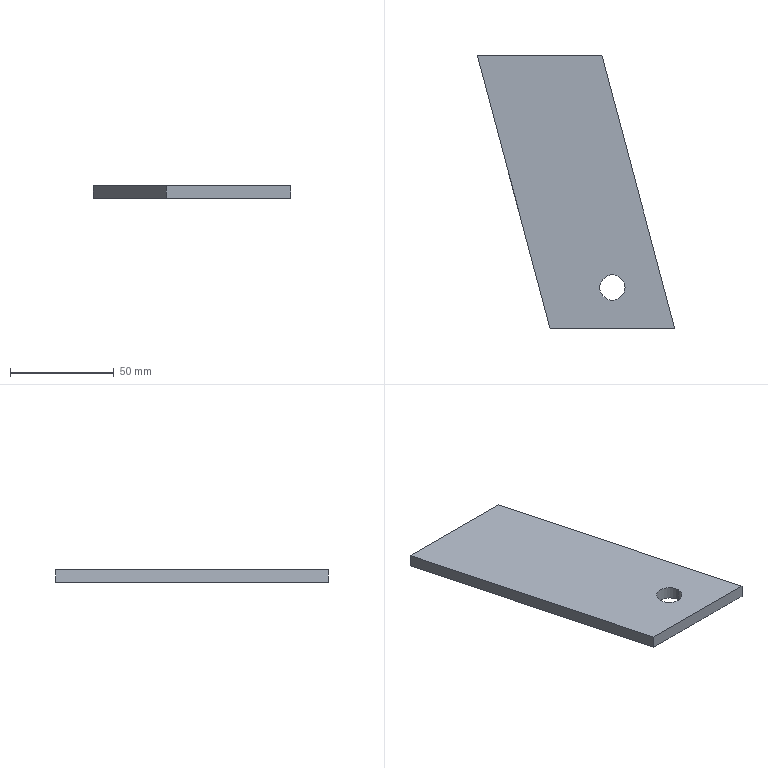Part | SolidWorks | features Extrusion 1, ICE 1 | 1 solid | 8 faces | box 95 x 131 x 6 mm | volume 46459 mm3 | plane 6 | cylinder 2 | commonest cylinder face diameters 12.2 x2
STEP:
#1=CARTESIAN_POINT('',(41.1,-147.5,-3.));
#2=VERTEX_POINT('',#1);
#3=CARTESIAN_POINT('',(28.9,-147.5,-3.));
#4=VERTEX_POINT('',#3);
#5=CARTESIAN_POINT('',(35.,-147.5,-3.));
#6=DIRECTION('',(0.,0.,-1.));
#7=DIRECTION('',(-1.,0.,0.));
#8=AXIS2_PLACEMENT_3D('',#5,#6,#7);
#9=CIRCLE('',#8,6.1);
#10=EDGE_CURVE('',#2,#4,#9,.T.);
#11=ORIENTED_EDGE('',*,*,#10,.T.);
#12=CARTESIAN_POINT('',(28.9,-147.5,3.));
#13=VERTEX_POINT('',#12);
#14=CARTESIAN_POINT('',(28.9,-147.5,-15.));
#15=DIRECTION('',(0.,0.,1.));
#16=VECTOR('',#15,1000.);
#17=LINE('',#14,#16);
#18=EDGE_CURVE('',#4,#13,#17,.T.);
#19=ORIENTED_EDGE('',*,*,#18,.T.);
#20=CARTESIAN_POINT('',(41.1,-147.5,3.));
#21=VERTEX_POINT('',#20);
#22=CARTESIAN_POINT('',(35.,-147.5,3.));
#23=DIRECTION('',(0.,0.,-1.));
#24=DIRECTION('',(-1.,0.,0.));
#25=AXIS2_PLACEMENT_3D('',#22,#23,#24);
#26=CIRCLE('',#25,6.1);
#27=EDGE_CURVE('',#21,#13,#26,.T.);
#28=ORIENTED_EDGE('',*,*,#27,.F.);
#29=CARTESIAN_POINT('',(41.1,-147.5,-15.));
#30=DIRECTION('',(0.,0.,1.));
#31=VECTOR('',#30,1000.);
#32=LINE('',#29,#31);
#33=EDGE_CURVE('',#2,#21,#32,.T.);
#34=ORIENTED_EDGE('',*,*,#33,.F.);
#35=EDGE_LOOP('',(#11,#19,#28,#34));
#36=FACE_OUTER_BOUND('',#35,.T.);
#37=CARTESIAN_POINT('',(35.,-147.5,-15.));
#38=DIRECTION('',(0.,0.,1.));
#39=DIRECTION('',(1.,0.,0.));
#40=AXIS2_PLACEMENT_3D('',#37,#38,#39);
#41=CYLINDRICAL_SURFACE('',#40,6.1);
#42=ADVANCED_FACE('',(#36),#41,.F.);
#43=CARTESIAN_POINT('',(-30.,-36.,3.));
#44=VERTEX_POINT('',#43);
#45=CARTESIAN_POINT('',(5.,-167.,3.));
#46=VERTEX_POINT('',#45);
#47=CARTESIAN_POINT('',(5.,-167.,3.));
#48=DIRECTION('',(0.2581,-0.9661,0.));
#49=VECTOR('',#48,1000.);
#50=LINE('',#47,#49);
#51=EDGE_CURVE('',#44,#46,#50,.T.);
#52=ORIENTED_EDGE('',*,*,#51,.F.);
#53=CARTESIAN_POINT('',(-30.,-36.,-3.));
#54=VERTEX_POINT('',#53);
#55=CARTESIAN_POINT('',(-30.,-36.,-3.));
#56=DIRECTION('',(0.,0.,1.));
#57=VECTOR('',#56,1000.);
#58=LINE('',#55,#57);
#59=EDGE_CURVE('',#54,#44,#58,.T.);
#60=ORIENTED_EDGE('',*,*,#59,.F.);
#61=CARTESIAN_POINT('',(5.,-167.,-3.));
#62=VERTEX_POINT('',#61);
#63=CARTESIAN_POINT('',(5.,-167.,-3.));
#64=DIRECTION('',(0.2581,-0.9661,0.));
#65=VECTOR('',#64,1000.);
#66=LINE('',#63,#65);
#67=EDGE_CURVE('',#54,#62,#66,.T.);
#68=ORIENTED_EDGE('',*,*,#67,.T.);
#69=CARTESIAN_POINT('',(5.,-167.,-3.));
#70=DIRECTION('',(0.,0.,1.));
#71=VECTOR('',#70,1000.);
#72=LINE('',#69,#71);
#73=EDGE_CURVE('',#62,#46,#72,.T.);
#74=ORIENTED_EDGE('',*,*,#73,.T.);
#75=EDGE_LOOP('',(#52,#60,#68,#74));
#76=FACE_OUTER_BOUND('',#75,.T.);
#77=CARTESIAN_POINT('',(5.,-167.,-3.));
#78=DIRECTION('',(-0.9661,-0.2581,0.));
#79=DIRECTION('',(0.2581,-0.9661,0.));
#80=AXIS2_PLACEMENT_3D('',#77,#78,#79);
#81=PLANE('',#80);
#82=ADVANCED_FACE('',(#76),#81,.T.);
#83=CARTESIAN_POINT('',(30.,-36.,3.));
#84=VERTEX_POINT('',#83);
#85=CARTESIAN_POINT('',(-30.,-36.,3.));
#86=DIRECTION('',(-1.,0.,0.));
#87=VECTOR('',#86,1000.);
#88=LINE('',#85,#87);
#89=EDGE_CURVE('',#84,#44,#88,.T.);
#90=ORIENTED_EDGE('',*,*,#89,.F.);
#91=CARTESIAN_POINT('',(30.,-36.,-3.));
#92=VERTEX_POINT('',#91);
#93=CARTESIAN_POINT('',(30.,-36.,-3.));
#94=DIRECTION('',(0.,0.,1.));
#95=VECTOR('',#94,1000.);
#96=LINE('',#93,#95);
#97=EDGE_CURVE('',#92,#84,#96,.T.);
#98=ORIENTED_EDGE('',*,*,#97,.F.);
#99=CARTESIAN_POINT('',(-30.,-36.,-3.));
#100=DIRECTION('',(-1.,0.,0.));
#101=VECTOR('',#100,1000.);
#102=LINE('',#99,#101);
#103=EDGE_CURVE('',#92,#54,#102,.T.);
#104=ORIENTED_EDGE('',*,*,#103,.T.);
#105=ORIENTED_EDGE('',*,*,#59,.T.);
#106=EDGE_LOOP('',(#90,#98,#104,#105));
#107=FACE_OUTER_BOUND('',#106,.T.);
#108=CARTESIAN_POINT('',(-30.,-36.,-3.));
#109=DIRECTION('',(0.,1.,0.));
#110=DIRECTION('',(0.,0.,1.));
#111=AXIS2_PLACEMENT_3D('',#108,#109,#110);
#112=PLANE('',#111);
#113=ADVANCED_FACE('',(#107),#112,.T.);
#114=CARTESIAN_POINT('',(65.,-167.,3.));
#115=VERTEX_POINT('',#114);
#116=CARTESIAN_POINT('',(30.,-36.,3.));
#117=DIRECTION('',(-0.2581,0.9661,0.));
#118=VECTOR('',#117,1000.);
#119=LINE('',#116,#118);
#120=EDGE_CURVE('',#115,#84,#119,.T.);
#121=ORIENTED_EDGE('',*,*,#120,.F.);
#122=CARTESIAN_POINT('',(65.,-167.,-3.));
#123=VERTEX_POINT('',#122);
#124=CARTESIAN_POINT('',(65.,-167.,-3.));
#125=DIRECTION('',(0.,0.,1.));
#126=VECTOR('',#125,1000.);
#127=LINE('',#124,#126);
#128=EDGE_CURVE('',#123,#115,#127,.T.);
#129=ORIENTED_EDGE('',*,*,#128,.F.);
#130=CARTESIAN_POINT('',(30.,-36.,-3.));
#131=DIRECTION('',(-0.2581,0.9661,0.));
#132=VECTOR('',#131,1000.);
#133=LINE('',#130,#132);
#134=EDGE_CURVE('',#123,#92,#133,.T.);
#135=ORIENTED_EDGE('',*,*,#134,.T.);
#136=ORIENTED_EDGE('',*,*,#97,.T.);
#137=EDGE_LOOP('',(#121,#129,#135,#136));
#138=FACE_OUTER_BOUND('',#137,.T.);
#139=CARTESIAN_POINT('',(30.,-36.,-3.));
#140=DIRECTION('',(0.9661,0.2581,0.));
#141=DIRECTION('',(-0.2581,0.9661,0.));
#142=AXIS2_PLACEMENT_3D('',#139,#140,#141);
#143=PLANE('',#142);
#144=ADVANCED_FACE('',(#138),#143,.T.);
#145=CARTESIAN_POINT('',(65.,-167.,3.));
#146=DIRECTION('',(1.,0.,0.));
#147=VECTOR('',#146,1000.);
#148=LINE('',#145,#147);
#149=EDGE_CURVE('',#46,#115,#148,.T.);
#150=ORIENTED_EDGE('',*,*,#149,.F.);
#151=ORIENTED_EDGE('',*,*,#73,.F.);
#152=CARTESIAN_POINT('',(65.,-167.,-3.));
#153=DIRECTION('',(1.,0.,0.));
#154=VECTOR('',#153,1000.);
#155=LINE('',#152,#154);
#156=EDGE_CURVE('',#62,#123,#155,.T.);
#157=ORIENTED_EDGE('',*,*,#156,.T.);
#158=ORIENTED_EDGE('',*,*,#128,.T.);
#159=EDGE_LOOP('',(#150,#151,#157,#158));
#160=FACE_OUTER_BOUND('',#159,.T.);
#161=CARTESIAN_POINT('',(65.,-167.,-3.));
#162=DIRECTION('',(0.,-1.,0.));
#163=DIRECTION('',(0.,0.,-1.));
#164=AXIS2_PLACEMENT_3D('',#161,#162,#163);
#165=PLANE('',#164);
#166=ADVANCED_FACE('',(#160),#165,.T.);
#167=ORIENTED_EDGE('',*,*,#10,.F.);
#168=CARTESIAN_POINT('',(35.,-147.5,-3.));
#169=DIRECTION('',(0.,0.,-1.));
#170=DIRECTION('',(-1.,0.,0.));
#171=AXIS2_PLACEMENT_3D('',#168,#169,#170);
#172=CIRCLE('',#171,6.1);
#173=EDGE_CURVE('',#4,#2,#172,.T.);
#174=ORIENTED_EDGE('',*,*,#173,.F.);
#175=EDGE_LOOP('',(#167,#174));
#176=FACE_BOUND('',#175,.T.);
#177=ORIENTED_EDGE('',*,*,#67,.F.);
#178=ORIENTED_EDGE('',*,*,#103,.F.);
#179=ORIENTED_EDGE('',*,*,#134,.F.);
#180=ORIENTED_EDGE('',*,*,#156,.F.);
#181=EDGE_LOOP('',(#177,#178,#179,#180));
#182=FACE_OUTER_BOUND('',#181,.T.);
#183=CARTESIAN_POINT('',(0.,0.,-3.));
#184=DIRECTION('',(0.,0.,-1.));
#185=DIRECTION('',(-1.,0.,0.));
#186=AXIS2_PLACEMENT_3D('',#183,#184,#185);
#187=PLANE('',#186);
#188=ADVANCED_FACE('',(#176,#182),#187,.T.);
#189=ORIENTED_EDGE('',*,*,#27,.T.);
#190=CARTESIAN_POINT('',(35.,-147.5,3.));
#191=DIRECTION('',(0.,0.,-1.));
#192=DIRECTION('',(-1.,0.,0.));
#193=AXIS2_PLACEMENT_3D('',#190,#191,#192);
#194=CIRCLE('',#193,6.1);
#195=EDGE_CURVE('',#13,#21,#194,.T.);
#196=ORIENTED_EDGE('',*,*,#195,.T.);
#197=EDGE_LOOP('',(#189,#196));
#198=FACE_BOUND('',#197,.T.);
#199=ORIENTED_EDGE('',*,*,#51,.T.);
#200=ORIENTED_EDGE('',*,*,#149,.T.);
#201=ORIENTED_EDGE('',*,*,#120,.T.);
#202=ORIENTED_EDGE('',*,*,#89,.T.);
#203=EDGE_LOOP('',(#199,#200,#201,#202));
#204=FACE_OUTER_BOUND('',#203,.T.);
#205=CARTESIAN_POINT('',(0.,0.,3.));
#206=DIRECTION('',(0.,0.,-1.));
#207=DIRECTION('',(-1.,0.,0.));
#208=AXIS2_PLACEMENT_3D('',#205,#206,#207);
#209=PLANE('',#208);
#210=ADVANCED_FACE('',(#198,#204),#209,.F.);
#211=ORIENTED_EDGE('',*,*,#18,.F.);
#212=ORIENTED_EDGE('',*,*,#173,.T.);
#213=ORIENTED_EDGE('',*,*,#33,.T.);
#214=ORIENTED_EDGE('',*,*,#195,.F.);
#215=EDGE_LOOP('',(#211,#212,#213,#214));
#216=FACE_OUTER_BOUND('',#215,.T.);
#217=CARTESIAN_POINT('',(35.,-147.5,-15.));
#218=DIRECTION('',(0.,0.,1.));
#219=DIRECTION('',(1.,0.,0.));
#220=AXIS2_PLACEMENT_3D('',#217,#218,#219);
#221=CYLINDRICAL_SURFACE('',#220,6.1);
#222=ADVANCED_FACE('',(#216),#221,.F.);
#223=CLOSED_SHELL('',(#42,#82,#113,#144,#166,#188,#210,#222));
#224=MANIFOLD_SOLID_BREP('',#223);
#225=CARTESIAN_POINT('',(0.,0.,0.));
#226=DIRECTION('',(0.,0.,1.));
#227=DIRECTION('',(1.,0.,0.));
#228=AXIS2_PLACEMENT_3D('',#225,#226,#227);
#229=(LENGTH_UNIT()NAMED_UNIT(*)SI_UNIT(.MILLI.,.METRE.));
#230=UNCERTAINTY_MEASURE_WITH_UNIT(LENGTH_MEASURE(0.00001),#229,'','');
#231=(NAMED_UNIT(*)PLANE_ANGLE_UNIT()SI_UNIT($,.RADIAN.));
#232=(NAMED_UNIT(*)SI_UNIT($,.STERADIAN.)SOLID_ANGLE_UNIT());
#233=(GEOMETRIC_REPRESENTATION_CONTEXT(3)GLOBAL_UNCERTAINTY_ASSIGNED_CONTEXT((#230))GLOBAL_UNIT_ASSIGNED_CONTEXT((#229,#231,#232))REPRESENTATION_CONTEXT('',''));
#234=ADVANCED_BREP_SHAPE_REPRESENTATION('',(#224,#228),#233);